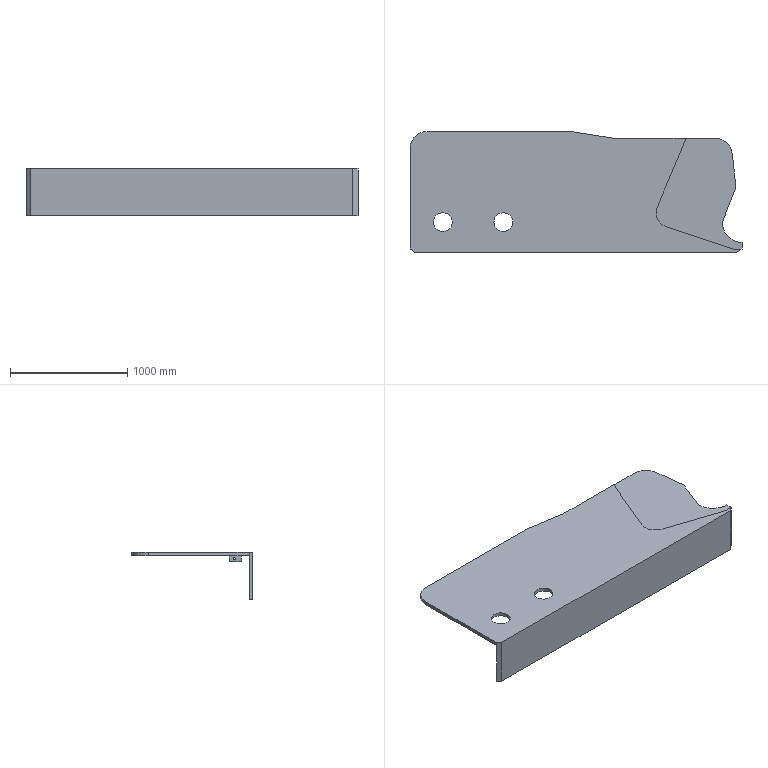Part | NX | features 掩护梁侧护板左 2 | 1 solid | 46 faces | box 2828 x 1030 x 405 mm | volume 109946345 mm3 | plane 36 | cylinder 10 | commonest cylinder face diameters 20 x4 160.33 x2 291.509 x2 250.37 x1 334.604 x1
STEP:
#1=CARTESIAN_POINT('',(589.52,-402.895,0.));
#2=VERTEX_POINT('',#1);
#3=CARTESIAN_POINT('',(589.52,-320.895,0.));
#4=VERTEX_POINT('',#3);
#5=CARTESIAN_POINT('',(589.52,-320.895,0.));
#6=DIRECTION('',(0.,1.,0.));
#7=VECTOR('',#6,1000.);
#8=LINE('',#5,#7);
#9=EDGE_CURVE('',#2,#4,#8,.T.);
#10=ORIENTED_EDGE('',*,*,#9,.F.);
#11=CARTESIAN_POINT('',(507.52,-402.895,0.));
#12=VERTEX_POINT('',#11);
#13=CARTESIAN_POINT('',(589.52,-402.895,0.));
#14=DIRECTION('',(1.,0.,0.));
#15=VECTOR('',#14,1000.);
#16=LINE('',#13,#15);
#17=EDGE_CURVE('',#12,#2,#16,.T.);
#18=ORIENTED_EDGE('',*,*,#17,.F.);
#19=CARTESIAN_POINT('',(507.52,-320.895,0.));
#20=VERTEX_POINT('',#19);
#21=CARTESIAN_POINT('',(507.52,-320.895,0.));
#22=DIRECTION('',(0.,-1.,0.));
#23=VECTOR('',#22,1000.);
#24=LINE('',#21,#23);
#25=EDGE_CURVE('',#20,#12,#24,.T.);
#26=ORIENTED_EDGE('',*,*,#25,.F.);
#27=CARTESIAN_POINT('',(482.52,-320.895,0.));
#28=VERTEX_POINT('',#27);
#29=CARTESIAN_POINT('',(482.52,-320.895,0.));
#30=DIRECTION('',(1.,0.,0.));
#31=VECTOR('',#30,1000.);
#32=LINE('',#29,#31);
#33=EDGE_CURVE('',#28,#20,#32,.T.);
#34=ORIENTED_EDGE('',*,*,#33,.F.);
#35=CARTESIAN_POINT('',(482.52,-422.895,0.));
#36=VERTEX_POINT('',#35);
#37=CARTESIAN_POINT('',(482.52,-422.895,0.));
#38=DIRECTION('',(0.,1.,0.));
#39=VECTOR('',#38,1000.);
#40=LINE('',#37,#39);
#41=EDGE_CURVE('',#36,#28,#40,.T.);
#42=ORIENTED_EDGE('',*,*,#41,.F.);
#43=CARTESIAN_POINT('',(614.52,-422.895,0.));
#44=VERTEX_POINT('',#43);
#45=CARTESIAN_POINT('',(614.52,-422.895,0.));
#46=DIRECTION('',(-1.,0.,0.));
#47=VECTOR('',#46,1000.);
#48=LINE('',#45,#47);
#49=EDGE_CURVE('',#44,#36,#48,.T.);
#50=ORIENTED_EDGE('',*,*,#49,.F.);
#51=CARTESIAN_POINT('',(614.52,-320.895,0.));
#52=VERTEX_POINT('',#51);
#53=CARTESIAN_POINT('',(614.52,-320.895,0.));
#54=DIRECTION('',(0.,-1.,0.));
#55=VECTOR('',#54,1000.);
#56=LINE('',#53,#55);
#57=EDGE_CURVE('',#52,#44,#56,.T.);
#58=ORIENTED_EDGE('',*,*,#57,.F.);
#59=CARTESIAN_POINT('',(589.52,-320.895,0.));
#60=DIRECTION('',(1.,0.,0.));
#61=VECTOR('',#60,1000.);
#62=LINE('',#59,#61);
#63=EDGE_CURVE('',#4,#52,#62,.T.);
#64=ORIENTED_EDGE('',*,*,#63,.F.);
#65=EDGE_LOOP('',(#10,#18,#26,#34,#42,#50,#58,#64));
#66=FACE_BOUND('',#65,.T.);
#67=CARTESIAN_POINT('',(-541.636,-260.046,0.));
#68=VERTEX_POINT('',#67);
#69=CARTESIAN_POINT('',(-621.801,-260.046,0.));
#70=DIRECTION('',(0.,0.,1.));
#71=DIRECTION('',(1.,0.,0.));
#72=AXIS2_PLACEMENT_3D('',#69,#70,#71);
#73=CIRCLE('',#72,80.165);
#74=EDGE_CURVE('',#68,#68,#73,.T.);
#75=ORIENTED_EDGE('',*,*,#74,.T.);
#76=EDGE_LOOP('',(#75));
#77=FACE_BOUND('',#76,.T.);
#78=CARTESIAN_POINT('',(-1056.636,-260.046,0.));
#79=VERTEX_POINT('',#78);
#80=CARTESIAN_POINT('',(-1136.801,-260.046,0.));
#81=DIRECTION('',(0.,0.,1.));
#82=DIRECTION('',(1.,0.,0.));
#83=AXIS2_PLACEMENT_3D('',#80,#81,#82);
#84=CIRCLE('',#83,80.165);
#85=EDGE_CURVE('',#79,#79,#84,.T.);
#86=ORIENTED_EDGE('',*,*,#85,.T.);
#87=EDGE_LOOP('',(#86));
#88=FACE_BOUND('',#87,.T.);
#89=CARTESIAN_POINT('',(-1416.65,-488.395,0.));
#90=VERTEX_POINT('',#89);
#91=CARTESIAN_POINT('',(1410.992,-488.395,0.));
#92=VERTEX_POINT('',#91);
#93=CARTESIAN_POINT('',(1410.992,-488.395,0.));
#94=DIRECTION('',(1.,0.,0.));
#95=VECTOR('',#94,1000.);
#96=LINE('',#93,#95);
#97=EDGE_CURVE('',#90,#92,#96,.T.);
#98=ORIENTED_EDGE('',*,*,#97,.F.);
#99=CARTESIAN_POINT('',(-1416.65,366.699,0.));
#100=VERTEX_POINT('',#99);
#101=CARTESIAN_POINT('',(-1416.65,366.699,0.));
#102=DIRECTION('',(0.,-1.,0.));
#103=VECTOR('',#102,1000.);
#104=LINE('',#101,#103);
#105=EDGE_CURVE('',#100,#90,#104,.T.);
#106=ORIENTED_EDGE('',*,*,#105,.F.);
#107=CARTESIAN_POINT('',(-1270.895,512.454,0.));
#108=VERTEX_POINT('',#107);
#109=CARTESIAN_POINT('',(-1270.895,366.699,0.));
#110=DIRECTION('',(0.,0.,1.));
#111=DIRECTION('',(1.,0.,0.));
#112=AXIS2_PLACEMENT_3D('',#109,#110,#111);
#113=CIRCLE('',#112,145.755);
#114=EDGE_CURVE('',#108,#100,#113,.T.);
#115=ORIENTED_EDGE('',*,*,#114,.F.);
#116=CARTESIAN_POINT('',(-51.414,512.454,0.));
#117=VERTEX_POINT('',#116);
#118=CARTESIAN_POINT('',(-51.414,512.454,0.));
#119=DIRECTION('',(-1.,0.,0.));
#120=VECTOR('',#119,1000.);
#121=LINE('',#118,#120);
#122=EDGE_CURVE('',#117,#108,#121,.T.);
#123=ORIENTED_EDGE('',*,*,#122,.F.);
#124=CARTESIAN_POINT('',(324.663,454.152,0.));
#125=VERTEX_POINT('',#124);
#126=CARTESIAN_POINT('',(324.663,454.152,0.));
#127=DIRECTION('',(-0.9882,0.1532,0.));
#128=VECTOR('',#127,1000.);
#129=LINE('',#126,#128);
#130=EDGE_CURVE('',#125,#117,#129,.T.);
#131=ORIENTED_EDGE('',*,*,#130,.F.);
#132=CARTESIAN_POINT('',(1182.944,454.152,0.));
#133=VERTEX_POINT('',#132);
#134=CARTESIAN_POINT('',(935.041,454.152,0.));
#135=DIRECTION('',(-1.,0.,0.));
#136=VECTOR('',#135,1000.);
#137=LINE('',#134,#136);
#138=EDGE_CURVE('',#133,#125,#137,.T.);
#139=ORIENTED_EDGE('',*,*,#138,.F.);
#140=CARTESIAN_POINT('',(1327.809,324.481,0.));
#141=VERTEX_POINT('',#140);
#142=CARTESIAN_POINT('',(1182.944,308.397,0.));
#143=DIRECTION('',(0.,0.,1.));
#144=DIRECTION('',(1.,0.,0.));
#145=AXIS2_PLACEMENT_3D('',#142,#143,#144);
#146=CIRCLE('',#145,145.755);
#147=EDGE_CURVE('',#141,#133,#146,.T.);
#148=ORIENTED_EDGE('',*,*,#147,.F.);
#149=CARTESIAN_POINT('',(1359.76,36.697,0.));
#150=VERTEX_POINT('',#149);
#151=CARTESIAN_POINT('',(1359.76,36.697,0.));
#152=DIRECTION('',(-0.1103,0.9939,0.));
#153=VECTOR('',#152,1000.);
#154=LINE('',#151,#153);
#155=EDGE_CURVE('',#150,#141,#154,.T.);
#156=ORIENTED_EDGE('',*,*,#155,.F.);
#157=CARTESIAN_POINT('',(1243.69,-260.046,0.));
#158=VERTEX_POINT('',#157);
#159=CARTESIAN_POINT('',(1243.69,-260.046,0.));
#160=DIRECTION('',(0.3643,0.9313,0.));
#161=VECTOR('',#160,1000.);
#162=LINE('',#159,#161);
#163=EDGE_CURVE('',#158,#150,#162,.T.);
#164=ORIENTED_EDGE('',*,*,#163,.F.);
#165=CARTESIAN_POINT('',(1410.992,-432.474,0.));
#166=VERTEX_POINT('',#165);
#167=CARTESIAN_POINT('',(1410.913,-265.172,0.));
#168=DIRECTION('',(0.,0.,-1.));
#169=DIRECTION('',(1.,0.,0.));
#170=AXIS2_PLACEMENT_3D('',#167,#168,#169);
#171=CIRCLE('',#170,167.302);
#172=EDGE_CURVE('',#166,#158,#171,.T.);
#173=ORIENTED_EDGE('',*,*,#172,.F.);
#174=CARTESIAN_POINT('',(1410.992,-488.395,0.));
#175=DIRECTION('',(0.,1.,0.));
#176=VECTOR('',#175,1000.);
#177=LINE('',#174,#176);
#178=EDGE_CURVE('',#92,#166,#177,.T.);
#179=ORIENTED_EDGE('',*,*,#178,.F.);
#180=EDGE_LOOP('',(#98,#106,#115,#123,#131,#139,#148,#156,#164,#173,#179));
#181=FACE_BOUND('',#180,.T.);
#182=CARTESIAN_POINT('',(-870.51,-402.895,0.));
#183=VERTEX_POINT('',#182);
#184=CARTESIAN_POINT('',(-870.51,-320.895,0.));
#185=VERTEX_POINT('',#184);
#186=CARTESIAN_POINT('',(-870.51,-320.895,0.));
#187=DIRECTION('',(0.,1.,0.));
#188=VECTOR('',#187,1000.);
#189=LINE('',#186,#188);
#190=EDGE_CURVE('',#183,#185,#189,.T.);
#191=ORIENTED_EDGE('',*,*,#190,.F.);
#192=CARTESIAN_POINT('',(-952.51,-402.895,0.));
#193=VERTEX_POINT('',#192);
#194=CARTESIAN_POINT('',(-870.51,-402.895,0.));
#195=DIRECTION('',(1.,0.,0.));
#196=VECTOR('',#195,1000.);
#197=LINE('',#194,#196);
#198=EDGE_CURVE('',#193,#183,#197,.T.);
#199=ORIENTED_EDGE('',*,*,#198,.F.);
#200=CARTESIAN_POINT('',(-952.51,-320.895,0.));
#201=VERTEX_POINT('',#200);
#202=CARTESIAN_POINT('',(-952.51,-320.895,0.));
#203=DIRECTION('',(0.,-1.,0.));
#204=VECTOR('',#203,1000.);
#205=LINE('',#202,#204);
#206=EDGE_CURVE('',#201,#193,#205,.T.);
#207=ORIENTED_EDGE('',*,*,#206,.F.);
#208=CARTESIAN_POINT('',(-977.51,-320.895,0.));
#209=VERTEX_POINT('',#208);
#210=CARTESIAN_POINT('',(-977.51,-320.895,0.));
#211=DIRECTION('',(1.,0.,0.));
#212=VECTOR('',#211,1000.);
#213=LINE('',#210,#212);
#214=EDGE_CURVE('',#209,#201,#213,.T.);
#215=ORIENTED_EDGE('',*,*,#214,.F.);
#216=CARTESIAN_POINT('',(-977.51,-422.895,0.));
#217=VERTEX_POINT('',#216);
#218=CARTESIAN_POINT('',(-977.51,-422.895,0.));
#219=DIRECTION('',(0.,1.,0.));
#220=VECTOR('',#219,1000.);
#221=LINE('',#218,#220);
#222=EDGE_CURVE('',#217,#209,#221,.T.);
#223=ORIENTED_EDGE('',*,*,#222,.F.);
#224=CARTESIAN_POINT('',(-845.51,-422.895,0.));
#225=VERTEX_POINT('',#224);
#226=CARTESIAN_POINT('',(-845.51,-422.895,0.));
#227=DIRECTION('',(-1.,0.,0.));
#228=VECTOR('',#227,1000.);
#229=LINE('',#226,#228);
#230=EDGE_CURVE('',#225,#217,#229,.T.);
#231=ORIENTED_EDGE('',*,*,#230,.F.);
#232=CARTESIAN_POINT('',(-845.51,-320.895,0.));
#233=VERTEX_POINT('',#232);
#234=CARTESIAN_POINT('',(-845.51,-320.895,0.));
#235=DIRECTION('',(0.,-1.,0.));
#236=VECTOR('',#235,1000.);
#237=LINE('',#234,#236);
#238=EDGE_CURVE('',#233,#225,#237,.T.);
#239=ORIENTED_EDGE('',*,*,#238,.F.);
#240=CARTESIAN_POINT('',(-870.51,-320.895,0.));
#241=DIRECTION('',(1.,0.,0.));
#242=VECTOR('',#241,1000.);
#243=LINE('',#240,#242);
#244=EDGE_CURVE('',#185,#233,#243,.T.);
#245=ORIENTED_EDGE('',*,*,#244,.F.);
#246=EDGE_LOOP('',(#191,#199,#207,#215,#223,#231,#239,#245));
#247=FACE_BOUND('',#246,.T.);
#248=CARTESIAN_POINT('',(-1270.895,366.699,0.));
#249=DIRECTION('',(0.,0.,1.));
#250=DIRECTION('',(1.,0.,0.));
#251=AXIS2_PLACEMENT_3D('',#248,#249,#250);
#252=PLANE('',#251);
#253=ADVANCED_FACE('',(#66,#77,#88,#181,#247),#252,.F.);
#254=CARTESIAN_POINT('',(1410.992,-488.395,25.));
#255=VERTEX_POINT('',#254);
#256=CARTESIAN_POINT('',(1410.992,-432.474,25.));
#257=VERTEX_POINT('',#256);
#258=CARTESIAN_POINT('',(1410.992,-488.395,25.));
#259=DIRECTION('',(0.,1.,0.));
#260=VECTOR('',#259,1000.);
#261=LINE('',#258,#260);
#262=EDGE_CURVE('',#255,#257,#261,.T.);
#263=ORIENTED_EDGE('',*,*,#262,.F.);
#264=CARTESIAN_POINT('',(1410.992,-488.395,30.));
#265=DIRECTION('',(0.,0.,-1.));
#266=VECTOR('',#265,1000.);
#267=LINE('',#264,#266);
#268=EDGE_CURVE('',#255,#92,#267,.T.);
#269=ORIENTED_EDGE('',*,*,#268,.T.);
#270=ORIENTED_EDGE('',*,*,#178,.T.);
#271=CARTESIAN_POINT('',(1410.992,-432.474,30.));
#272=DIRECTION('',(0.,0.,-1.));
#273=VECTOR('',#272,1000.);
#274=LINE('',#271,#273);
#275=EDGE_CURVE('',#257,#166,#274,.T.);
#276=ORIENTED_EDGE('',*,*,#275,.F.);
#277=EDGE_LOOP('',(#263,#269,#270,#276));
#278=FACE_BOUND('',#277,.T.);
#279=CARTESIAN_POINT('',(1410.992,-488.395,30.));
#280=DIRECTION('',(-1.,0.,0.));
#281=DIRECTION('',(0.,0.,1.));
#282=AXIS2_PLACEMENT_3D('',#279,#280,#281);
#283=PLANE('',#282);
#284=ADVANCED_FACE('',(#278),#283,.F.);
#285=CARTESIAN_POINT('',(1243.69,-260.046,25.));
#286=VERTEX_POINT('',#285);
#287=CARTESIAN_POINT('',(1410.913,-265.172,25.));
#288=DIRECTION('',(0.,0.,1.));
#289=DIRECTION('',(1.,0.,0.));
#290=AXIS2_PLACEMENT_3D('',#287,#288,#289);
#291=CIRCLE('',#290,167.302);
#292=EDGE_CURVE('',#257,#286,#291,.F.);
#293=ORIENTED_EDGE('',*,*,#292,.F.);
#294=ORIENTED_EDGE('',*,*,#275,.T.);
#295=ORIENTED_EDGE('',*,*,#172,.T.);
#296=CARTESIAN_POINT('',(1243.69,-260.046,30.));
#297=DIRECTION('',(0.,0.,-1.));
#298=VECTOR('',#297,1000.);
#299=LINE('',#296,#298);
#300=EDGE_CURVE('',#286,#158,#299,.T.);
#301=ORIENTED_EDGE('',*,*,#300,.F.);
#302=EDGE_LOOP('',(#293,#294,#295,#301));
#303=FACE_BOUND('',#302,.T.);
#304=CARTESIAN_POINT('',(1410.913,-265.172,30.));
#305=DIRECTION('',(0.,0.,-1.));
#306=DIRECTION('',(-1.,0.,0.));
#307=AXIS2_PLACEMENT_3D('',#304,#305,#306);
#308=CYLINDRICAL_SURFACE('',#307,167.302);
#309=ADVANCED_FACE('',(#303),#308,.F.);
#310=CARTESIAN_POINT('',(1359.76,36.697,25.));
#311=VERTEX_POINT('',#310);
#312=CARTESIAN_POINT('',(1243.69,-260.046,25.));
#313=DIRECTION('',(0.3643,0.9313,0.));
#314=VECTOR('',#313,1000.);
#315=LINE('',#312,#314);
#316=EDGE_CURVE('',#286,#311,#315,.T.);
#317=ORIENTED_EDGE('',*,*,#316,.F.);
#318=ORIENTED_EDGE('',*,*,#300,.T.);
#319=ORIENTED_EDGE('',*,*,#163,.T.);
#320=CARTESIAN_POINT('',(1359.76,36.697,30.));
#321=DIRECTION('',(0.,0.,-1.));
#322=VECTOR('',#321,1000.);
#323=LINE('',#320,#322);
#324=EDGE_CURVE('',#311,#150,#323,.T.);
#325=ORIENTED_EDGE('',*,*,#324,.F.);
#326=EDGE_LOOP('',(#317,#318,#319,#325));
#327=FACE_BOUND('',#326,.T.);
#328=CARTESIAN_POINT('',(1243.69,-260.046,30.));
#329=DIRECTION('',(-0.9313,0.3643,0.));
#330=DIRECTION('',(-0.3643,-0.9313,0.));
#331=AXIS2_PLACEMENT_3D('',#328,#329,#330);
#332=PLANE('',#331);
#333=ADVANCED_FACE('',(#327),#332,.F.);
#334=CARTESIAN_POINT('',(1327.809,324.481,25.));
#335=VERTEX_POINT('',#334);
#336=CARTESIAN_POINT('',(1359.76,36.697,25.));
#337=DIRECTION('',(-0.1103,0.9939,0.));
#338=VECTOR('',#337,1000.);
#339=LINE('',#336,#338);
#340=EDGE_CURVE('',#311,#335,#339,.T.);
#341=ORIENTED_EDGE('',*,*,#340,.F.);
#342=ORIENTED_EDGE('',*,*,#324,.T.);
#343=ORIENTED_EDGE('',*,*,#155,.T.);
#344=CARTESIAN_POINT('',(1327.809,324.481,30.));
#345=DIRECTION('',(0.,0.,-1.));
#346=VECTOR('',#345,1000.);
#347=LINE('',#344,#346);
#348=EDGE_CURVE('',#335,#141,#347,.T.);
#349=ORIENTED_EDGE('',*,*,#348,.F.);
#350=EDGE_LOOP('',(#341,#342,#343,#349));
#351=FACE_BOUND('',#350,.T.);
#352=CARTESIAN_POINT('',(1359.76,36.697,30.));
#353=DIRECTION('',(-0.9939,-0.1103,0.));
#354=DIRECTION('',(0.1103,-0.9939,0.));
#355=AXIS2_PLACEMENT_3D('',#352,#353,#354);
#356=PLANE('',#355);
#357=ADVANCED_FACE('',(#351),#356,.F.);
#358=CARTESIAN_POINT('',(1182.944,454.152,25.));
#359=VERTEX_POINT('',#358);
#360=CARTESIAN_POINT('',(1182.944,308.397,25.));
#361=DIRECTION('',(0.,0.,1.));
#362=DIRECTION('',(1.,0.,0.));
#363=AXIS2_PLACEMENT_3D('',#360,#361,#362);
#364=CIRCLE('',#363,145.755);
#365=EDGE_CURVE('',#335,#359,#364,.T.);
#366=ORIENTED_EDGE('',*,*,#365,.F.);
#367=ORIENTED_EDGE('',*,*,#348,.T.);
#368=ORIENTED_EDGE('',*,*,#147,.T.);
#369=CARTESIAN_POINT('',(1182.944,454.152,30.));
#370=DIRECTION('',(0.,0.,-1.));
#371=VECTOR('',#370,1000.);
#372=LINE('',#369,#371);
#373=EDGE_CURVE('',#359,#133,#372,.T.);
#374=ORIENTED_EDGE('',*,*,#373,.F.);
#375=EDGE_LOOP('',(#366,#367,#368,#374));
#376=FACE_BOUND('',#375,.T.);
#377=CARTESIAN_POINT('',(1182.944,308.397,30.));
#378=DIRECTION('',(0.,0.,-1.));
#379=DIRECTION('',(-1.,0.,0.));
#380=AXIS2_PLACEMENT_3D('',#377,#378,#379);
#381=CYLINDRICAL_SURFACE('',#380,145.755);
#382=ADVANCED_FACE('',(#376),#381,.T.);
#383=CARTESIAN_POINT('',(1337.166,-488.395,30.));
#384=VERTEX_POINT('',#383);
#385=CARTESIAN_POINT('',(1410.992,-488.395,30.));
#386=VERTEX_POINT('',#385);
#387=CARTESIAN_POINT('',(1337.166,-488.395,30.));
#388=DIRECTION('',(1.,0.,0.));
#389=VECTOR('',#388,1000.);
#390=LINE('',#387,#389);
#391=EDGE_CURVE('',#384,#386,#390,.T.);
#392=ORIENTED_EDGE('',*,*,#391,.F.);
#393=CARTESIAN_POINT('',(764.685,-299.875,30.));
#394=VERTEX_POINT('',#393);
#395=CARTESIAN_POINT('',(764.685,-299.875,30.));
#396=DIRECTION('',(0.9498,-0.3128,0.));
#397=VECTOR('',#396,1000.);
#398=LINE('',#395,#397);
#399=EDGE_CURVE('',#394,#384,#398,.T.);
#400=ORIENTED_EDGE('',*,*,#399,.F.);
#401=CARTESIAN_POINT('',(688.438,-132.458,30.));
#402=VERTEX_POINT('',#401);
#403=CARTESIAN_POINT('',(803.841,-180.971,30.));
#404=DIRECTION('',(0.,0.,1.));
#405=DIRECTION('',(1.,0.,0.));
#406=AXIS2_PLACEMENT_3D('',#403,#404,#405);
#407=CIRCLE('',#406,125.185);
#408=EDGE_CURVE('',#402,#394,#407,.T.);
#409=ORIENTED_EDGE('',*,*,#408,.F.);
#410=CARTESIAN_POINT('',(935.041,454.152,30.));
#411=VERTEX_POINT('',#410);
#412=CARTESIAN_POINT('',(935.041,454.152,30.));
#413=DIRECTION('',(-0.3875,-0.9219,0.));
#414=VECTOR('',#413,1000.);
#415=LINE('',#412,#414);
#416=EDGE_CURVE('',#411,#402,#415,.T.);
#417=ORIENTED_EDGE('',*,*,#416,.F.);
#418=CARTESIAN_POINT('',(324.663,454.152,30.));
#419=VERTEX_POINT('',#418);
#420=CARTESIAN_POINT('',(1182.944,454.152,30.));
#421=DIRECTION('',(-1.,0.,0.));
#422=VECTOR('',#421,1000.);
#423=LINE('',#420,#422);
#424=EDGE_CURVE('',#411,#419,#423,.T.);
#425=ORIENTED_EDGE('',*,*,#424,.T.);
#426=CARTESIAN_POINT('',(-51.414,512.454,30.));
#427=VERTEX_POINT('',#426);
#428=CARTESIAN_POINT('',(324.663,454.152,30.));
#429=DIRECTION('',(-0.9882,0.1532,0.));
#430=VECTOR('',#429,1000.);
#431=LINE('',#428,#430);
#432=EDGE_CURVE('',#419,#427,#431,.T.);
#433=ORIENTED_EDGE('',*,*,#432,.T.);
#434=CARTESIAN_POINT('',(-1270.895,512.454,30.));
#435=VERTEX_POINT('',#434);
#436=CARTESIAN_POINT('',(-51.414,512.454,30.));
#437=DIRECTION('',(-1.,0.,0.));
#438=VECTOR('',#437,1000.);
#439=LINE('',#436,#438);
#440=EDGE_CURVE('',#427,#435,#439,.T.);
#441=ORIENTED_EDGE('',*,*,#440,.T.);
#442=CARTESIAN_POINT('',(-1416.65,366.699,30.));
#443=VERTEX_POINT('',#442);
#444=CARTESIAN_POINT('',(-1270.895,366.699,30.));
#445=DIRECTION('',(0.,0.,1.));
#446=DIRECTION('',(1.,0.,0.));
#447=AXIS2_PLACEMENT_3D('',#444,#445,#446);
#448=CIRCLE('',#447,145.755);
#449=EDGE_CURVE('',#435,#443,#448,.T.);
#450=ORIENTED_EDGE('',*,*,#449,.T.);
#451=CARTESIAN_POINT('',(-1416.65,-488.395,30.));
#452=VERTEX_POINT('',#451);
#453=CARTESIAN_POINT('',(-1416.65,366.699,30.));
#454=DIRECTION('',(0.,-1.,0.));
#455=VECTOR('',#454,1000.);
#456=LINE('',#453,#455);
#457=EDGE_CURVE('',#443,#452,#456,.T.);
#458=ORIENTED_EDGE('',*,*,#457,.T.);
#459=CARTESIAN_POINT('',(-1381.422,-517.546,30.));
#460=VERTEX_POINT('',#459);
#461=CARTESIAN_POINT('',(-1381.422,-517.546,30.));
#462=DIRECTION('',(0.7704,-0.6375,0.));
#463=VECTOR('',#462,1000.);
#464=LINE('',#461,#463);
#465=EDGE_CURVE('',#452,#460,#464,.T.);
#466=ORIENTED_EDGE('',*,*,#465,.T.);
#467=CARTESIAN_POINT('',(1367.913,-517.546,30.));
#468=VERTEX_POINT('',#467);
#469=CARTESIAN_POINT('',(1367.913,-517.546,30.));
#470=DIRECTION('',(1.,0.,0.));
#471=VECTOR('',#470,1000.);
#472=LINE('',#469,#471);
#473=EDGE_CURVE('',#460,#468,#472,.T.);
#474=ORIENTED_EDGE('',*,*,#473,.T.);
#475=CARTESIAN_POINT('',(1410.992,-488.395,30.));
#476=DIRECTION('',(0.8282,0.5604,0.));
#477=VECTOR('',#476,1000.);
#478=LINE('',#475,#477);
#479=EDGE_CURVE('',#468,#386,#478,.T.);
#480=ORIENTED_EDGE('',*,*,#479,.T.);
#481=EDGE_LOOP('',(#392,#400,#409,#417,#425,#433,#441,#450,#458,#466,#474,#480));
#482=FACE_BOUND('',#481,.T.);
#483=CARTESIAN_POINT('',(-1056.636,-260.046,30.));
#484=VERTEX_POINT('',#483);
#485=CARTESIAN_POINT('',(-1136.801,-260.046,30.));
#486=DIRECTION('',(0.,0.,1.));
#487=DIRECTION('',(1.,0.,0.));
#488=AXIS2_PLACEMENT_3D('',#485,#486,#487);
#489=CIRCLE('',#488,80.165);
#490=EDGE_CURVE('',#484,#484,#489,.T.);
#491=ORIENTED_EDGE('',*,*,#490,.F.);
#492=EDGE_LOOP('',(#491));
#493=FACE_BOUND('',#492,.T.);
#494=CARTESIAN_POINT('',(-541.636,-260.046,30.));
#495=VERTEX_POINT('',#494);
#496=CARTESIAN_POINT('',(-621.801,-260.046,30.));
#497=DIRECTION('',(0.,0.,1.));
#498=DIRECTION('',(1.,0.,0.));
#499=AXIS2_PLACEMENT_3D('',#496,#497,#498);
#500=CIRCLE('',#499,80.165);
#501=EDGE_CURVE('',#495,#495,#500,.T.);
#502=ORIENTED_EDGE('',*,*,#501,.F.);
#503=EDGE_LOOP('',(#502));
#504=FACE_BOUND('',#503,.T.);
#505=CARTESIAN_POINT('',(-1270.895,366.699,30.));
#506=DIRECTION('',(0.,0.,1.));
#507=DIRECTION('',(1.,0.,0.));
#508=AXIS2_PLACEMENT_3D('',#505,#506,#507);
#509=PLANE('',#508);
#510=ADVANCED_FACE('',(#482,#493,#504),#509,.T.);
#511=ORIENTED_EDGE('',*,*,#114,.T.);
#512=CARTESIAN_POINT('',(-1416.65,366.699,30.));
#513=DIRECTION('',(0.,0.,-1.));
#514=VECTOR('',#513,1000.);
#515=LINE('',#512,#514);
#516=EDGE_CURVE('',#443,#100,#515,.T.);
#517=ORIENTED_EDGE('',*,*,#516,.F.);
#518=ORIENTED_EDGE('',*,*,#449,.F.);
#519=CARTESIAN_POINT('',(-1270.895,512.454,30.));
#520=DIRECTION('',(0.,0.,-1.));
#521=VECTOR('',#520,1000.);
#522=LINE('',#519,#521);
#523=EDGE_CURVE('',#435,#108,#522,.T.);
#524=ORIENTED_EDGE('',*,*,#523,.T.);
#525=EDGE_LOOP('',(#511,#517,#518,#524));
#526=FACE_BOUND('',#525,.T.);
#527=CARTESIAN_POINT('',(-1270.895,366.699,30.));
#528=DIRECTION('',(0.,0.,-1.));
#529=DIRECTION('',(-1.,0.,0.));
#530=AXIS2_PLACEMENT_3D('',#527,#528,#529);
#531=CYLINDRICAL_SURFACE('',#530,145.755);
#532=ADVANCED_FACE('',(#526),#531,.T.);
#533=ORIENTED_EDGE('',*,*,#105,.T.);
#534=CARTESIAN_POINT('',(-1416.65,-488.395,30.));
#535=DIRECTION('',(0.,0.,-1.));
#536=VECTOR('',#535,1000.);
#537=LINE('',#534,#536);
#538=EDGE_CURVE('',#452,#90,#537,.T.);
#539=ORIENTED_EDGE('',*,*,#538,.F.);
#540=ORIENTED_EDGE('',*,*,#457,.F.);
#541=ORIENTED_EDGE('',*,*,#516,.T.);
#542=EDGE_LOOP('',(#533,#539,#540,#541));
#543=FACE_BOUND('',#542,.T.);
#544=CARTESIAN_POINT('',(-1416.65,366.699,30.));
#545=DIRECTION('',(1.,0.,0.));
#546=DIRECTION('',(0.,0.,-1.));
#547=AXIS2_PLACEMENT_3D('',#544,#545,#546);
#548=PLANE('',#547);
#549=ADVANCED_FACE('',(#543),#548,.F.);
#550=ORIENTED_EDGE('',*,*,#538,.T.);
#551=CARTESIAN_POINT('',(-1416.65,-488.395,-375.));
#552=VERTEX_POINT('',#551);
#553=CARTESIAN_POINT('',(-1416.65,-488.395,-375.));
#554=DIRECTION('',(0.,0.,1.));
#555=VECTOR('',#554,1000.);
#556=LINE('',#553,#555);
#557=EDGE_CURVE('',#552,#90,#556,.T.);
#558=ORIENTED_EDGE('',*,*,#557,.F.);
#559=CARTESIAN_POINT('',(-1381.422,-517.546,-375.));
#560=VERTEX_POINT('',#559);
#561=CARTESIAN_POINT('',(-1416.65,-488.395,-375.));
#562=DIRECTION('',(-0.7704,0.6375,0.));
#563=VECTOR('',#562,1000.);
#564=LINE('',#561,#563);
#565=EDGE_CURVE('',#560,#552,#564,.T.);
#566=ORIENTED_EDGE('',*,*,#565,.F.);
#567=CARTESIAN_POINT('',(-1381.422,-517.546,30.));
#568=DIRECTION('',(0.,0.,-1.));
#569=VECTOR('',#568,1000.);
#570=LINE('',#567,#569);
#571=EDGE_CURVE('',#460,#560,#570,.T.);
#572=ORIENTED_EDGE('',*,*,#571,.F.);
#573=ORIENTED_EDGE('',*,*,#465,.F.);
#574=EDGE_LOOP('',(#550,#558,#566,#572,#573));
#575=FACE_BOUND('',#574,.T.);
#576=CARTESIAN_POINT('',(-1381.422,-517.546,30.));
#577=DIRECTION('',(0.6375,0.7704,0.));
#578=DIRECTION('',(-0.7704,0.6375,0.));
#579=AXIS2_PLACEMENT_3D('',#576,#577,#578);
#580=PLANE('',#579);
#581=ADVANCED_FACE('',(#575),#580,.F.);
#582=ORIENTED_EDGE('',*,*,#571,.T.);
#583=CARTESIAN_POINT('',(1367.913,-517.546,-375.));
#584=VERTEX_POINT('',#583);
#585=CARTESIAN_POINT('',(-1381.422,-517.546,-375.));
#586=DIRECTION('',(-1.,0.,0.));
#587=VECTOR('',#586,1000.);
#588=LINE('',#585,#587);
#589=EDGE_CURVE('',#584,#560,#588,.T.);
#590=ORIENTED_EDGE('',*,*,#589,.F.);
#591=CARTESIAN_POINT('',(1367.913,-517.546,30.));
#592=DIRECTION('',(0.,0.,-1.));
#593=VECTOR('',#592,1000.);
#594=LINE('',#591,#593);
#595=EDGE_CURVE('',#468,#584,#594,.T.);
#596=ORIENTED_EDGE('',*,*,#595,.F.);
#597=ORIENTED_EDGE('',*,*,#473,.F.);
#598=EDGE_LOOP('',(#582,#590,#596,#597));
#599=FACE_BOUND('',#598,.T.);
#600=CARTESIAN_POINT('',(1367.913,-517.546,30.));
#601=DIRECTION('',(0.,1.,0.));
#602=DIRECTION('',(-1.,0.,0.));
#603=AXIS2_PLACEMENT_3D('',#600,#601,#602);
#604=PLANE('',#603);
#605=ADVANCED_FACE('',(#599),#604,.F.);
#606=ORIENTED_EDGE('',*,*,#595,.T.);
#607=CARTESIAN_POINT('',(1410.992,-488.395,-375.));
#608=VERTEX_POINT('',#607);
#609=CARTESIAN_POINT('',(1367.913,-517.546,-375.));
#610=DIRECTION('',(-0.8282,-0.5604,0.));
#611=VECTOR('',#610,1000.);
#612=LINE('',#609,#611);
#613=EDGE_CURVE('',#608,#584,#612,.T.);
#614=ORIENTED_EDGE('',*,*,#613,.F.);
#615=CARTESIAN_POINT('',(1410.992,-488.395,-375.));
#616=DIRECTION('',(0.,0.,1.));
#617=VECTOR('',#616,1000.);
#618=LINE('',#615,#617);
#619=EDGE_CURVE('',#608,#92,#618,.T.);
#620=ORIENTED_EDGE('',*,*,#619,.T.);
#621=ORIENTED_EDGE('',*,*,#268,.F.);
#622=CARTESIAN_POINT('',(1410.992,-488.395,30.));
#623=DIRECTION('',(0.,0.,-1.));
#624=VECTOR('',#623,1000.);
#625=LINE('',#622,#624);
#626=EDGE_CURVE('',#386,#255,#625,.T.);
#627=ORIENTED_EDGE('',*,*,#626,.F.);
#628=ORIENTED_EDGE('',*,*,#479,.F.);
#629=EDGE_LOOP('',(#606,#614,#620,#621,#627,#628));
#630=FACE_BOUND('',#629,.T.);
#631=CARTESIAN_POINT('',(1410.992,-488.395,30.));
#632=DIRECTION('',(-0.5604,0.8282,0.));
#633=DIRECTION('',(-0.8282,-0.5604,0.));
#634=AXIS2_PLACEMENT_3D('',#631,#632,#633);
#635=PLANE('',#634);
#636=ADVANCED_FACE('',(#630),#635,.F.);
#637=ORIENTED_EDGE('',*,*,#424,.F.);
#638=CARTESIAN_POINT('',(935.041,454.152,25.));
#639=VERTEX_POINT('',#638);
#640=CARTESIAN_POINT('',(935.041,454.152,25.));
#641=DIRECTION('',(0.,0.,1.));
#642=VECTOR('',#641,1000.);
#643=LINE('',#640,#642);
#644=EDGE_CURVE('',#639,#411,#643,.T.);
#645=ORIENTED_EDGE('',*,*,#644,.F.);
#646=CARTESIAN_POINT('',(935.041,454.152,25.));
#647=DIRECTION('',(-1.,0.,0.));
#648=VECTOR('',#647,1000.);
#649=LINE('',#646,#648);
#650=EDGE_CURVE('',#359,#639,#649,.T.);
#651=ORIENTED_EDGE('',*,*,#650,.F.);
#652=ORIENTED_EDGE('',*,*,#373,.T.);
#653=ORIENTED_EDGE('',*,*,#138,.T.);
#654=CARTESIAN_POINT('',(324.663,454.152,30.));
#655=DIRECTION('',(0.,0.,-1.));
#656=VECTOR('',#655,1000.);
#657=LINE('',#654,#656);
#658=EDGE_CURVE('',#419,#125,#657,.T.);
#659=ORIENTED_EDGE('',*,*,#658,.F.);
#660=EDGE_LOOP('',(#637,#645,#651,#652,#653,#659));
#661=FACE_BOUND('',#660,.T.);
#662=CARTESIAN_POINT('',(935.041,454.152,30.));
#663=DIRECTION('',(0.,-1.,0.));
#664=DIRECTION('',(1.,0.,0.));
#665=AXIS2_PLACEMENT_3D('',#662,#663,#664);
#666=PLANE('',#665);
#667=ADVANCED_FACE('',(#661),#666,.F.);
#668=ORIENTED_EDGE('',*,*,#130,.T.);
#669=CARTESIAN_POINT('',(-51.414,512.454,30.));
#670=DIRECTION('',(0.,0.,-1.));
#671=VECTOR('',#670,1000.);
#672=LINE('',#669,#671);
#673=EDGE_CURVE('',#427,#117,#672,.T.);
#674=ORIENTED_EDGE('',*,*,#673,.F.);
#675=ORIENTED_EDGE('',*,*,#432,.F.);
#676=ORIENTED_EDGE('',*,*,#658,.T.);
#677=EDGE_LOOP('',(#668,#674,#675,#676));
#678=FACE_BOUND('',#677,.T.);
#679=CARTESIAN_POINT('',(324.663,454.152,30.));
#680=DIRECTION('',(-0.1532,-0.9882,0.));
#681=DIRECTION('',(0.9882,-0.1532,0.));
#682=AXIS2_PLACEMENT_3D('',#679,#680,#681);
#683=PLANE('',#682);
#684=ADVANCED_FACE('',(#678),#683,.F.);
#685=ORIENTED_EDGE('',*,*,#122,.T.);
#686=ORIENTED_EDGE('',*,*,#523,.F.);
#687=ORIENTED_EDGE('',*,*,#440,.F.);
#688=ORIENTED_EDGE('',*,*,#673,.T.);
#689=EDGE_LOOP('',(#685,#686,#687,#688));
#690=FACE_BOUND('',#689,.T.);
#691=CARTESIAN_POINT('',(-51.414,512.454,30.));
#692=DIRECTION('',(0.,-1.,0.));
#693=DIRECTION('',(0.,0.,-1.));
#694=AXIS2_PLACEMENT_3D('',#691,#692,#693);
#695=PLANE('',#694);
#696=ADVANCED_FACE('',(#690),#695,.F.);
#697=ORIENTED_EDGE('',*,*,#490,.T.);
#698=EDGE_LOOP('',(#697));
#699=FACE_BOUND('',#698,.T.);
#700=ORIENTED_EDGE('',*,*,#85,.F.);
#701=EDGE_LOOP('',(#700));
#702=FACE_BOUND('',#701,.T.);
#703=CARTESIAN_POINT('',(-1136.801,-260.046,30.));
#704=DIRECTION('',(0.,0.,-1.));
#705=DIRECTION('',(-1.,0.,0.));
#706=AXIS2_PLACEMENT_3D('',#703,#704,#705);
#707=CYLINDRICAL_SURFACE('',#706,80.165);
#708=ADVANCED_FACE('',(#699,#702),#707,.F.);
#709=ORIENTED_EDGE('',*,*,#501,.T.);
#710=EDGE_LOOP('',(#709));
#711=FACE_BOUND('',#710,.T.);
#712=ORIENTED_EDGE('',*,*,#74,.F.);
#713=EDGE_LOOP('',(#712));
#714=FACE_BOUND('',#713,.T.);
#715=CARTESIAN_POINT('',(-621.801,-260.046,30.));
#716=DIRECTION('',(0.,0.,-1.));
#717=DIRECTION('',(-1.,0.,0.));
#718=AXIS2_PLACEMENT_3D('',#715,#716,#717);
#719=CYLINDRICAL_SURFACE('',#718,80.165);
#720=ADVANCED_FACE('',(#711,#714),#719,.F.);
#721=ORIENTED_EDGE('',*,*,#292,.T.);
#722=ORIENTED_EDGE('',*,*,#316,.T.);
#723=ORIENTED_EDGE('',*,*,#340,.T.);
#724=ORIENTED_EDGE('',*,*,#365,.T.);
#725=ORIENTED_EDGE('',*,*,#650,.T.);
#726=CARTESIAN_POINT('',(688.438,-132.458,25.));
#727=VERTEX_POINT('',#726);
#728=CARTESIAN_POINT('',(935.041,454.152,25.));
#729=DIRECTION('',(-0.3875,-0.9219,0.));
#730=VECTOR('',#729,1000.);
#731=LINE('',#728,#730);
#732=EDGE_CURVE('',#639,#727,#731,.T.);
#733=ORIENTED_EDGE('',*,*,#732,.T.);
#734=CARTESIAN_POINT('',(764.685,-299.875,25.));
#735=VERTEX_POINT('',#734);
#736=CARTESIAN_POINT('',(803.841,-180.971,25.));
#737=DIRECTION('',(0.,0.,1.));
#738=DIRECTION('',(1.,0.,0.));
#739=AXIS2_PLACEMENT_3D('',#736,#737,#738);
#740=CIRCLE('',#739,125.185);
#741=EDGE_CURVE('',#727,#735,#740,.T.);
#742=ORIENTED_EDGE('',*,*,#741,.T.);
#743=CARTESIAN_POINT('',(1337.166,-488.395,25.));
#744=VERTEX_POINT('',#743);
#745=CARTESIAN_POINT('',(764.685,-299.875,25.));
#746=DIRECTION('',(0.9498,-0.3128,0.));
#747=VECTOR('',#746,1000.);
#748=LINE('',#745,#747);
#749=EDGE_CURVE('',#735,#744,#748,.T.);
#750=ORIENTED_EDGE('',*,*,#749,.T.);
#751=CARTESIAN_POINT('',(1337.166,-488.395,25.));
#752=DIRECTION('',(1.,0.,0.));
#753=VECTOR('',#752,1000.);
#754=LINE('',#751,#753);
#755=EDGE_CURVE('',#744,#255,#754,.T.);
#756=ORIENTED_EDGE('',*,*,#755,.T.);
#757=ORIENTED_EDGE('',*,*,#262,.T.);
#758=EDGE_LOOP('',(#721,#722,#723,#724,#725,#733,#742,#750,#756,#757));
#759=FACE_BOUND('',#758,.T.);
#760=CARTESIAN_POINT('',(1182.944,308.397,25.));
#761=DIRECTION('',(0.,0.,1.));
#762=DIRECTION('',(1.,0.,0.));
#763=AXIS2_PLACEMENT_3D('',#760,#761,#762);
#764=PLANE('',#763);
#765=ADVANCED_FACE('',(#759),#764,.T.);
#766=ORIENTED_EDGE('',*,*,#391,.T.);
#767=ORIENTED_EDGE('',*,*,#626,.T.);
#768=ORIENTED_EDGE('',*,*,#755,.F.);
#769=CARTESIAN_POINT('',(1337.166,-488.395,25.));
#770=DIRECTION('',(0.,0.,1.));
#771=VECTOR('',#770,1000.);
#772=LINE('',#769,#771);
#773=EDGE_CURVE('',#744,#384,#772,.T.);
#774=ORIENTED_EDGE('',*,*,#773,.T.);
#775=EDGE_LOOP('',(#766,#767,#768,#774));
#776=FACE_BOUND('',#775,.T.);
#777=CARTESIAN_POINT('',(1337.166,-488.395,25.));
#778=DIRECTION('',(0.,-1.,0.));
#779=DIRECTION('',(0.,0.,-1.));
#780=AXIS2_PLACEMENT_3D('',#777,#778,#779);
#781=PLANE('',#780);
#782=ADVANCED_FACE('',(#776),#781,.F.);
#783=ORIENTED_EDGE('',*,*,#399,.T.);
#784=ORIENTED_EDGE('',*,*,#773,.F.);
#785=ORIENTED_EDGE('',*,*,#749,.F.);
#786=CARTESIAN_POINT('',(764.685,-299.875,25.));
#787=DIRECTION('',(0.,0.,1.));
#788=VECTOR('',#787,1000.);
#789=LINE('',#786,#788);
#790=EDGE_CURVE('',#735,#394,#789,.T.);
#791=ORIENTED_EDGE('',*,*,#790,.T.);
#792=EDGE_LOOP('',(#783,#784,#785,#791));
#793=FACE_BOUND('',#792,.T.);
#794=CARTESIAN_POINT('',(764.685,-299.875,25.));
#795=DIRECTION('',(-0.3128,-0.9498,0.));
#796=DIRECTION('',(0.9498,-0.3128,0.));
#797=AXIS2_PLACEMENT_3D('',#794,#795,#796);
#798=PLANE('',#797);
#799=ADVANCED_FACE('',(#793),#798,.F.);
#800=ORIENTED_EDGE('',*,*,#408,.T.);
#801=ORIENTED_EDGE('',*,*,#790,.F.);
#802=ORIENTED_EDGE('',*,*,#741,.F.);
#803=CARTESIAN_POINT('',(688.438,-132.458,25.));
#804=DIRECTION('',(0.,0.,1.));
#805=VECTOR('',#804,1000.);
#806=LINE('',#803,#805);
#807=EDGE_CURVE('',#727,#402,#806,.T.);
#808=ORIENTED_EDGE('',*,*,#807,.T.);
#809=EDGE_LOOP('',(#800,#801,#802,#808));
#810=FACE_BOUND('',#809,.T.);
#811=CARTESIAN_POINT('',(803.841,-180.971,25.));
#812=DIRECTION('',(0.,0.,1.));
#813=DIRECTION('',(1.,0.,0.));
#814=AXIS2_PLACEMENT_3D('',#811,#812,#813);
#815=CYLINDRICAL_SURFACE('',#814,125.185);
#816=ADVANCED_FACE('',(#810),#815,.F.);
#817=ORIENTED_EDGE('',*,*,#416,.T.);
#818=ORIENTED_EDGE('',*,*,#807,.F.);
#819=ORIENTED_EDGE('',*,*,#732,.F.);
#820=ORIENTED_EDGE('',*,*,#644,.T.);
#821=EDGE_LOOP('',(#817,#818,#819,#820));
#822=FACE_BOUND('',#821,.T.);
#823=CARTESIAN_POINT('',(935.041,454.152,25.));
#824=DIRECTION('',(-0.9219,0.3875,0.));
#825=DIRECTION('',(-0.3875,-0.9219,0.));
#826=AXIS2_PLACEMENT_3D('',#823,#824,#825);
#827=PLANE('',#826);
#828=ADVANCED_FACE('',(#822),#827,.F.);
#829=ORIENTED_EDGE('',*,*,#97,.T.);
#830=ORIENTED_EDGE('',*,*,#619,.F.);
#831=CARTESIAN_POINT('',(1410.992,-488.395,-375.));
#832=DIRECTION('',(1.,0.,0.));
#833=VECTOR('',#832,1000.);
#834=LINE('',#831,#833);
#835=EDGE_CURVE('',#552,#608,#834,.T.);
#836=ORIENTED_EDGE('',*,*,#835,.F.);
#837=ORIENTED_EDGE('',*,*,#557,.T.);
#838=EDGE_LOOP('',(#829,#830,#836,#837));
#839=FACE_BOUND('',#838,.T.);
#840=CARTESIAN_POINT('',(1410.992,-488.395,-375.));
#841=DIRECTION('',(0.,-1.,0.));
#842=DIRECTION('',(0.,0.,-1.));
#843=AXIS2_PLACEMENT_3D('',#840,#841,#842);
#844=PLANE('',#843);
#845=ADVANCED_FACE('',(#839),#844,.F.);
#846=ORIENTED_EDGE('',*,*,#613,.T.);
#847=ORIENTED_EDGE('',*,*,#589,.T.);
#848=ORIENTED_EDGE('',*,*,#565,.T.);
#849=ORIENTED_EDGE('',*,*,#835,.T.);
#850=EDGE_LOOP('',(#846,#847,#848,#849));
#851=FACE_BOUND('',#850,.T.);
#852=CARTESIAN_POINT('',(-144.576,-1541.031,-375.));
#853=DIRECTION('',(0.,0.,-1.));
#854=DIRECTION('',(-1.,0.,0.));
#855=AXIS2_PLACEMENT_3D('',#852,#853,#854);
#856=PLANE('',#855);
#857=ADVANCED_FACE('',(#851),#856,.T.);
#858=CARTESIAN_POINT('',(589.52,-361.895,-35.));
#859=VERTEX_POINT('',#858);
#860=CARTESIAN_POINT('',(589.52,-361.895,-25.));
#861=DIRECTION('',(1.,0.,0.));
#862=DIRECTION('',(0.,0.,-1.));
#863=AXIS2_PLACEMENT_3D('',#860,#861,#862);
#864=CIRCLE('',#863,10.);
#865=EDGE_CURVE('',#859,#859,#864,.T.);
#866=ORIENTED_EDGE('',*,*,#865,.T.);
#867=EDGE_LOOP('',(#866));
#868=FACE_BOUND('',#867,.T.);
#869=ORIENTED_EDGE('',*,*,#9,.T.);
#870=CARTESIAN_POINT('',(589.52,-320.895,-50.));
#871=VERTEX_POINT('',#870);
#872=CARTESIAN_POINT('',(589.52,-320.895,-50.));
#873=DIRECTION('',(0.,0.,1.));
#874=VECTOR('',#873,1000.);
#875=LINE('',#872,#874);
#876=EDGE_CURVE('',#871,#4,#875,.T.);
#877=ORIENTED_EDGE('',*,*,#876,.F.);
#878=CARTESIAN_POINT('',(589.52,-402.895,-50.));
#879=VERTEX_POINT('',#878);
#880=CARTESIAN_POINT('',(589.52,-320.895,-50.));
#881=DIRECTION('',(0.,1.,0.));
#882=VECTOR('',#881,1000.);
#883=LINE('',#880,#882);
#884=EDGE_CURVE('',#879,#871,#883,.T.);
#885=ORIENTED_EDGE('',*,*,#884,.F.);
#886=CARTESIAN_POINT('',(589.52,-402.895,-50.));
#887=DIRECTION('',(0.,0.,1.));
#888=VECTOR('',#887,1000.);
#889=LINE('',#886,#888);
#890=EDGE_CURVE('',#879,#2,#889,.T.);
#891=ORIENTED_EDGE('',*,*,#890,.T.);
#892=EDGE_LOOP('',(#869,#877,#885,#891));
#893=FACE_BOUND('',#892,.T.);
#894=CARTESIAN_POINT('',(589.52,-320.895,-50.));
#895=DIRECTION('',(1.,0.,0.));
#896=DIRECTION('',(0.,0.,-1.));
#897=AXIS2_PLACEMENT_3D('',#894,#895,#896);
#898=PLANE('',#897);
#899=ADVANCED_FACE('',(#868,#893),#898,.F.);
#900=ORIENTED_EDGE('',*,*,#63,.T.);
#901=CARTESIAN_POINT('',(614.52,-320.895,-50.));
#902=VERTEX_POINT('',#901);
#903=CARTESIAN_POINT('',(614.52,-320.895,-50.));
#904=DIRECTION('',(0.,0.,1.));
#905=VECTOR('',#904,1000.);
#906=LINE('',#903,#905);
#907=EDGE_CURVE('',#902,#52,#906,.T.);
#908=ORIENTED_EDGE('',*,*,#907,.F.);
#909=CARTESIAN_POINT('',(589.52,-320.895,-50.));
#910=DIRECTION('',(1.,0.,0.));
#911=VECTOR('',#910,1000.);
#912=LINE('',#909,#911);
#913=EDGE_CURVE('',#871,#902,#912,.T.);
#914=ORIENTED_EDGE('',*,*,#913,.F.);
#915=ORIENTED_EDGE('',*,*,#876,.T.);
#916=EDGE_LOOP('',(#900,#908,#914,#915));
#917=FACE_BOUND('',#916,.T.);
#918=CARTESIAN_POINT('',(589.52,-320.895,-50.));
#919=DIRECTION('',(0.,-1.,0.));
#920=DIRECTION('',(0.,0.,-1.));
#921=AXIS2_PLACEMENT_3D('',#918,#919,#920);
#922=PLANE('',#921);
#923=ADVANCED_FACE('',(#917),#922,.F.);
#924=CARTESIAN_POINT('',(614.52,-361.895,-35.));
#925=VERTEX_POINT('',#924);
#926=CARTESIAN_POINT('',(614.52,-361.895,-25.));
#927=DIRECTION('',(1.,0.,0.));
#928=DIRECTION('',(0.,0.,-1.));
#929=AXIS2_PLACEMENT_3D('',#926,#927,#928);
#930=CIRCLE('',#929,10.);
#931=EDGE_CURVE('',#925,#925,#930,.T.);
#932=ORIENTED_EDGE('',*,*,#931,.F.);
#933=EDGE_LOOP('',(#932));
#934=FACE_BOUND('',#933,.T.);
#935=ORIENTED_EDGE('',*,*,#57,.T.);
#936=CARTESIAN_POINT('',(614.52,-422.895,-50.));
#937=VERTEX_POINT('',#936);
#938=CARTESIAN_POINT('',(614.52,-422.895,-50.));
#939=DIRECTION('',(0.,0.,1.));
#940=VECTOR('',#939,1000.);
#941=LINE('',#938,#940);
#942=EDGE_CURVE('',#937,#44,#941,.T.);
#943=ORIENTED_EDGE('',*,*,#942,.F.);
#944=CARTESIAN_POINT('',(614.52,-320.895,-50.));
#945=DIRECTION('',(0.,-1.,0.));
#946=VECTOR('',#945,1000.);
#947=LINE('',#944,#946);
#948=EDGE_CURVE('',#902,#937,#947,.T.);
#949=ORIENTED_EDGE('',*,*,#948,.F.);
#950=ORIENTED_EDGE('',*,*,#907,.T.);
#951=EDGE_LOOP('',(#935,#943,#949,#950));
#952=FACE_BOUND('',#951,.T.);
#953=CARTESIAN_POINT('',(614.52,-320.895,-50.));
#954=DIRECTION('',(-1.,0.,0.));
#955=DIRECTION('',(0.,0.,1.));
#956=AXIS2_PLACEMENT_3D('',#953,#954,#955);
#957=PLANE('',#956);
#958=ADVANCED_FACE('',(#934,#952),#957,.F.);
#959=ORIENTED_EDGE('',*,*,#49,.T.);
#960=CARTESIAN_POINT('',(482.52,-422.895,-50.));
#961=VERTEX_POINT('',#960);
#962=CARTESIAN_POINT('',(482.52,-422.895,-50.));
#963=DIRECTION('',(0.,0.,1.));
#964=VECTOR('',#963,1000.);
#965=LINE('',#962,#964);
#966=EDGE_CURVE('',#961,#36,#965,.T.);
#967=ORIENTED_EDGE('',*,*,#966,.F.);
#968=CARTESIAN_POINT('',(614.52,-422.895,-50.));
#969=DIRECTION('',(-1.,0.,0.));
#970=VECTOR('',#969,1000.);
#971=LINE('',#968,#970);
#972=EDGE_CURVE('',#937,#961,#971,.T.);
#973=ORIENTED_EDGE('',*,*,#972,.F.);
#974=ORIENTED_EDGE('',*,*,#942,.T.);
#975=EDGE_LOOP('',(#959,#967,#973,#974));
#976=FACE_BOUND('',#975,.T.);
#977=CARTESIAN_POINT('',(614.52,-422.895,-50.));
#978=DIRECTION('',(0.,1.,0.));
#979=DIRECTION('',(0.,0.,1.));
#980=AXIS2_PLACEMENT_3D('',#977,#978,#979);
#981=PLANE('',#980);
#982=ADVANCED_FACE('',(#976),#981,.F.);
#983=CARTESIAN_POINT('',(482.52,-361.895,-35.));
#984=VERTEX_POINT('',#983);
#985=CARTESIAN_POINT('',(482.52,-361.895,-25.));
#986=DIRECTION('',(1.,0.,0.));
#987=DIRECTION('',(0.,0.,-1.));
#988=AXIS2_PLACEMENT_3D('',#985,#986,#987);
#989=CIRCLE('',#988,10.);
#990=EDGE_CURVE('',#984,#984,#989,.T.);
#991=ORIENTED_EDGE('',*,*,#990,.T.);
#992=EDGE_LOOP('',(#991));
#993=FACE_BOUND('',#992,.T.);
#994=ORIENTED_EDGE('',*,*,#41,.T.);
#995=CARTESIAN_POINT('',(482.52,-320.895,-50.));
#996=VERTEX_POINT('',#995);
#997=CARTESIAN_POINT('',(482.52,-320.895,-50.));
#998=DIRECTION('',(0.,0.,1.));
#999=VECTOR('',#998,1000.);
#1000=LINE('',#997,#999);
#1001=EDGE_CURVE('',#996,#28,#1000,.T.);
#1002=ORIENTED_EDGE('',*,*,#1001,.F.);
#1003=CARTESIAN_POINT('',(482.52,-422.895,-50.));
#1004=DIRECTION('',(0.,1.,0.));
#1005=VECTOR('',#1004,1000.);
#1006=LINE('',#1003,#1005);
#1007=EDGE_CURVE('',#961,#996,#1006,.T.);
#1008=ORIENTED_EDGE('',*,*,#1007,.F.);
#1009=ORIENTED_EDGE('',*,*,#966,.T.);
#1010=EDGE_LOOP('',(#994,#1002,#1008,#1009));
#1011=FACE_BOUND('',#1010,.T.);
#1012=CARTESIAN_POINT('',(482.52,-422.895,-50.));
#1013=DIRECTION('',(1.,0.,0.));
#1014=DIRECTION('',(0.,0.,-1.));
#1015=AXIS2_PLACEMENT_3D('',#1012,#1013,#1014);
#1016=PLANE('',#1015);
#1017=ADVANCED_FACE('',(#993,#1011),#1016,.F.);
#1018=ORIENTED_EDGE('',*,*,#33,.T.);
#1019=CARTESIAN_POINT('',(507.52,-320.895,-50.));
#1020=VERTEX_POINT('',#1019);
#1021=CARTESIAN_POINT('',(507.52,-320.895,-50.));
#1022=DIRECTION('',(0.,0.,1.));
#1023=VECTOR('',#1022,1000.);
#1024=LINE('',#1021,#1023);
#1025=EDGE_CURVE('',#1020,#20,#1024,.T.);
#1026=ORIENTED_EDGE('',*,*,#1025,.F.);
#1027=CARTESIAN_POINT('',(482.52,-320.895,-50.));
#1028=DIRECTION('',(1.,0.,0.));
#1029=VECTOR('',#1028,1000.);
#1030=LINE('',#1027,#1029);
#1031=EDGE_CURVE('',#996,#1020,#1030,.T.);
#1032=ORIENTED_EDGE('',*,*,#1031,.F.);
#1033=ORIENTED_EDGE('',*,*,#1001,.T.);
#1034=EDGE_LOOP('',(#1018,#1026,#1032,#1033));
#1035=FACE_BOUND('',#1034,.T.);
#1036=CARTESIAN_POINT('',(482.52,-320.895,-50.));
#1037=DIRECTION('',(0.,-1.,0.));
#1038=DIRECTION('',(0.,0.,-1.));
#1039=AXIS2_PLACEMENT_3D('',#1036,#1037,#1038);
#1040=PLANE('',#1039);
#1041=ADVANCED_FACE('',(#1035),#1040,.F.);
#1042=CARTESIAN_POINT('',(507.52,-361.895,-15.));
#1043=VERTEX_POINT('',#1042);
#1044=CARTESIAN_POINT('',(507.52,-361.895,-25.));
#1045=DIRECTION('',(-1.,0.,0.));
#1046=DIRECTION('',(0.,0.,1.));
#1047=AXIS2_PLACEMENT_3D('',#1044,#1045,#1046);
#1048=CIRCLE('',#1047,10.);
#1049=EDGE_CURVE('',#1043,#1043,#1048,.T.);
#1050=ORIENTED_EDGE('',*,*,#1049,.T.);
#1051=EDGE_LOOP('',(#1050));
#1052=FACE_BOUND('',#1051,.T.);
#1053=ORIENTED_EDGE('',*,*,#25,.T.);
#1054=CARTESIAN_POINT('',(507.52,-402.895,-50.));
#1055=VERTEX_POINT('',#1054);
#1056=CARTESIAN_POINT('',(507.52,-402.895,-50.));
#1057=DIRECTION('',(0.,0.,1.));
#1058=VECTOR('',#1057,1000.);
#1059=LINE('',#1056,#1058);
#1060=EDGE_CURVE('',#1055,#12,#1059,.T.);
#1061=ORIENTED_EDGE('',*,*,#1060,.F.);
#1062=CARTESIAN_POINT('',(507.52,-320.895,-50.));
#1063=DIRECTION('',(0.,-1.,0.));
#1064=VECTOR('',#1063,1000.);
#1065=LINE('',#1062,#1064);
#1066=EDGE_CURVE('',#1020,#1055,#1065,.T.);
#1067=ORIENTED_EDGE('',*,*,#1066,.F.);
#1068=ORIENTED_EDGE('',*,*,#1025,.T.);
#1069=EDGE_LOOP('',(#1053,#1061,#1067,#1068));
#1070=FACE_BOUND('',#1069,.T.);
#1071=CARTESIAN_POINT('',(507.52,-320.895,-50.));
#1072=DIRECTION('',(-1.,0.,0.));
#1073=DIRECTION('',(0.,0.,1.));
#1074=AXIS2_PLACEMENT_3D('',#1071,#1072,#1073);
#1075=PLANE('',#1074);
#1076=ADVANCED_FACE('',(#1052,#1070),#1075,.F.);
#1077=ORIENTED_EDGE('',*,*,#17,.T.);
#1078=ORIENTED_EDGE('',*,*,#890,.F.);
#1079=CARTESIAN_POINT('',(589.52,-402.895,-50.));
#1080=DIRECTION('',(1.,0.,0.));
#1081=VECTOR('',#1080,1000.);
#1082=LINE('',#1079,#1081);
#1083=EDGE_CURVE('',#1055,#879,#1082,.T.);
#1084=ORIENTED_EDGE('',*,*,#1083,.F.);
#1085=ORIENTED_EDGE('',*,*,#1060,.T.);
#1086=EDGE_LOOP('',(#1077,#1078,#1084,#1085));
#1087=FACE_BOUND('',#1086,.T.);
#1088=CARTESIAN_POINT('',(589.52,-402.895,-50.));
#1089=DIRECTION('',(0.,-1.,0.));
#1090=DIRECTION('',(0.,0.,-1.));
#1091=AXIS2_PLACEMENT_3D('',#1088,#1089,#1090);
#1092=PLANE('',#1091);
#1093=ADVANCED_FACE('',(#1087),#1092,.F.);
#1094=ORIENTED_EDGE('',*,*,#884,.T.);
#1095=ORIENTED_EDGE('',*,*,#913,.T.);
#1096=ORIENTED_EDGE('',*,*,#948,.T.);
#1097=ORIENTED_EDGE('',*,*,#972,.T.);
#1098=ORIENTED_EDGE('',*,*,#1007,.T.);
#1099=ORIENTED_EDGE('',*,*,#1031,.T.);
#1100=ORIENTED_EDGE('',*,*,#1066,.T.);
#1101=ORIENTED_EDGE('',*,*,#1083,.T.);
#1102=EDGE_LOOP('',(#1094,#1095,#1096,#1097,#1098,#1099,#1100,#1101));
#1103=FACE_BOUND('',#1102,.T.);
#1104=CARTESIAN_POINT('',(589.52,-402.895,-50.));
#1105=DIRECTION('',(0.,0.,-1.));
#1106=DIRECTION('',(-1.,0.,0.));
#1107=AXIS2_PLACEMENT_3D('',#1104,#1105,#1106);
#1108=PLANE('',#1107);
#1109=ADVANCED_FACE('',(#1103),#1108,.T.);
#1110=CARTESIAN_POINT('',(-870.51,-361.895,-35.));
#1111=VERTEX_POINT('',#1110);
#1112=CARTESIAN_POINT('',(-870.51,-361.895,-25.));
#1113=DIRECTION('',(1.,0.,0.));
#1114=DIRECTION('',(0.,0.,-1.));
#1115=AXIS2_PLACEMENT_3D('',#1112,#1113,#1114);
#1116=CIRCLE('',#1115,10.);
#1117=EDGE_CURVE('',#1111,#1111,#1116,.T.);
#1118=ORIENTED_EDGE('',*,*,#1117,.T.);
#1119=EDGE_LOOP('',(#1118));
#1120=FACE_BOUND('',#1119,.T.);
#1121=ORIENTED_EDGE('',*,*,#190,.T.);
#1122=CARTESIAN_POINT('',(-870.51,-320.895,-50.));
#1123=VERTEX_POINT('',#1122);
#1124=CARTESIAN_POINT('',(-870.51,-320.895,-50.));
#1125=DIRECTION('',(0.,0.,1.));
#1126=VECTOR('',#1125,1000.);
#1127=LINE('',#1124,#1126);
#1128=EDGE_CURVE('',#1123,#185,#1127,.T.);
#1129=ORIENTED_EDGE('',*,*,#1128,.F.);
#1130=CARTESIAN_POINT('',(-870.51,-402.895,-50.));
#1131=VERTEX_POINT('',#1130);
#1132=CARTESIAN_POINT('',(-870.51,-320.895,-50.));
#1133=DIRECTION('',(0.,1.,0.));
#1134=VECTOR('',#1133,1000.);
#1135=LINE('',#1132,#1134);
#1136=EDGE_CURVE('',#1131,#1123,#1135,.T.);
#1137=ORIENTED_EDGE('',*,*,#1136,.F.);
#1138=CARTESIAN_POINT('',(-870.51,-402.895,-50.));
#1139=DIRECTION('',(0.,0.,1.));
#1140=VECTOR('',#1139,1000.);
#1141=LINE('',#1138,#1140);
#1142=EDGE_CURVE('',#1131,#183,#1141,.T.);
#1143=ORIENTED_EDGE('',*,*,#1142,.T.);
#1144=EDGE_LOOP('',(#1121,#1129,#1137,#1143));
#1145=FACE_BOUND('',#1144,.T.);
#1146=CARTESIAN_POINT('',(-870.51,-320.895,-50.));
#1147=DIRECTION('',(1.,0.,0.));
#1148=DIRECTION('',(0.,0.,-1.));
#1149=AXIS2_PLACEMENT_3D('',#1146,#1147,#1148);
#1150=PLANE('',#1149);
#1151=ADVANCED_FACE('',(#1120,#1145),#1150,.F.);
#1152=ORIENTED_EDGE('',*,*,#244,.T.);
#1153=CARTESIAN_POINT('',(-845.51,-320.895,-50.));
#1154=VERTEX_POINT('',#1153);
#1155=CARTESIAN_POINT('',(-845.51,-320.895,-50.));
#1156=DIRECTION('',(0.,0.,1.));
#1157=VECTOR('',#1156,1000.);
#1158=LINE('',#1155,#1157);
#1159=EDGE_CURVE('',#1154,#233,#1158,.T.);
#1160=ORIENTED_EDGE('',*,*,#1159,.F.);
#1161=CARTESIAN_POINT('',(-870.51,-320.895,-50.));
#1162=DIRECTION('',(1.,0.,0.));
#1163=VECTOR('',#1162,1000.);
#1164=LINE('',#1161,#1163);
#1165=EDGE_CURVE('',#1123,#1154,#1164,.T.);
#1166=ORIENTED_EDGE('',*,*,#1165,.F.);
#1167=ORIENTED_EDGE('',*,*,#1128,.T.);
#1168=EDGE_LOOP('',(#1152,#1160,#1166,#1167));
#1169=FACE_BOUND('',#1168,.T.);
#1170=CARTESIAN_POINT('',(-870.51,-320.895,-50.));
#1171=DIRECTION('',(0.,-1.,0.));
#1172=DIRECTION('',(0.,0.,-1.));
#1173=AXIS2_PLACEMENT_3D('',#1170,#1171,#1172);
#1174=PLANE('',#1173);
#1175=ADVANCED_FACE('',(#1169),#1174,.F.);
#1176=CARTESIAN_POINT('',(-845.51,-361.895,-15.));
#1177=VERTEX_POINT('',#1176);
#1178=CARTESIAN_POINT('',(-845.51,-361.895,-25.));
#1179=DIRECTION('',(-1.,0.,0.));
#1180=DIRECTION('',(0.,0.,1.));
#1181=AXIS2_PLACEMENT_3D('',#1178,#1179,#1180);
#1182=CIRCLE('',#1181,10.);
#1183=EDGE_CURVE('',#1177,#1177,#1182,.T.);
#1184=ORIENTED_EDGE('',*,*,#1183,.T.);
#1185=EDGE_LOOP('',(#1184));
#1186=FACE_BOUND('',#1185,.T.);
#1187=ORIENTED_EDGE('',*,*,#238,.T.);
#1188=CARTESIAN_POINT('',(-845.51,-422.895,-50.));
#1189=VERTEX_POINT('',#1188);
#1190=CARTESIAN_POINT('',(-845.51,-422.895,-50.));
#1191=DIRECTION('',(0.,0.,1.));
#1192=VECTOR('',#1191,1000.);
#1193=LINE('',#1190,#1192);
#1194=EDGE_CURVE('',#1189,#225,#1193,.T.);
#1195=ORIENTED_EDGE('',*,*,#1194,.F.);
#1196=CARTESIAN_POINT('',(-845.51,-320.895,-50.));
#1197=DIRECTION('',(0.,-1.,0.));
#1198=VECTOR('',#1197,1000.);
#1199=LINE('',#1196,#1198);
#1200=EDGE_CURVE('',#1154,#1189,#1199,.T.);
#1201=ORIENTED_EDGE('',*,*,#1200,.F.);
#1202=ORIENTED_EDGE('',*,*,#1159,.T.);
#1203=EDGE_LOOP('',(#1187,#1195,#1201,#1202));
#1204=FACE_BOUND('',#1203,.T.);
#1205=CARTESIAN_POINT('',(-845.51,-320.895,-50.));
#1206=DIRECTION('',(-1.,0.,0.));
#1207=DIRECTION('',(0.,0.,1.));
#1208=AXIS2_PLACEMENT_3D('',#1205,#1206,#1207);
#1209=PLANE('',#1208);
#1210=ADVANCED_FACE('',(#1186,#1204),#1209,.F.);
#1211=ORIENTED_EDGE('',*,*,#230,.T.);
#1212=CARTESIAN_POINT('',(-977.51,-422.895,-50.));
#1213=VERTEX_POINT('',#1212);
#1214=CARTESIAN_POINT('',(-977.51,-422.895,-50.));
#1215=DIRECTION('',(0.,0.,1.));
#1216=VECTOR('',#1215,1000.);
#1217=LINE('',#1214,#1216);
#1218=EDGE_CURVE('',#1213,#217,#1217,.T.);
#1219=ORIENTED_EDGE('',*,*,#1218,.F.);
#1220=CARTESIAN_POINT('',(-845.51,-422.895,-50.));
#1221=DIRECTION('',(-1.,0.,0.));
#1222=VECTOR('',#1221,1000.);
#1223=LINE('',#1220,#1222);
#1224=EDGE_CURVE('',#1189,#1213,#1223,.T.);
#1225=ORIENTED_EDGE('',*,*,#1224,.F.);
#1226=ORIENTED_EDGE('',*,*,#1194,.T.);
#1227=EDGE_LOOP('',(#1211,#1219,#1225,#1226));
#1228=FACE_BOUND('',#1227,.T.);
#1229=CARTESIAN_POINT('',(-845.51,-422.895,-50.));
#1230=DIRECTION('',(0.,1.,0.));
#1231=DIRECTION('',(0.,0.,1.));
#1232=AXIS2_PLACEMENT_3D('',#1229,#1230,#1231);
#1233=PLANE('',#1232);
#1234=ADVANCED_FACE('',(#1228),#1233,.F.);
#1235=CARTESIAN_POINT('',(-977.51,-361.895,-35.));
#1236=VERTEX_POINT('',#1235);
#1237=CARTESIAN_POINT('',(-977.51,-361.895,-25.));
#1238=DIRECTION('',(1.,0.,0.));
#1239=DIRECTION('',(0.,0.,-1.));
#1240=AXIS2_PLACEMENT_3D('',#1237,#1238,#1239);
#1241=CIRCLE('',#1240,10.);
#1242=EDGE_CURVE('',#1236,#1236,#1241,.T.);
#1243=ORIENTED_EDGE('',*,*,#1242,.T.);
#1244=EDGE_LOOP('',(#1243));
#1245=FACE_BOUND('',#1244,.T.);
#1246=ORIENTED_EDGE('',*,*,#222,.T.);
#1247=CARTESIAN_POINT('',(-977.51,-320.895,-50.));
#1248=VERTEX_POINT('',#1247);
#1249=CARTESIAN_POINT('',(-977.51,-320.895,-50.));
#1250=DIRECTION('',(0.,0.,1.));
#1251=VECTOR('',#1250,1000.);
#1252=LINE('',#1249,#1251);
#1253=EDGE_CURVE('',#1248,#209,#1252,.T.);
#1254=ORIENTED_EDGE('',*,*,#1253,.F.);
#1255=CARTESIAN_POINT('',(-977.51,-422.895,-50.));
#1256=DIRECTION('',(0.,1.,0.));
#1257=VECTOR('',#1256,1000.);
#1258=LINE('',#1255,#1257);
#1259=EDGE_CURVE('',#1213,#1248,#1258,.T.);
#1260=ORIENTED_EDGE('',*,*,#1259,.F.);
#1261=ORIENTED_EDGE('',*,*,#1218,.T.);
#1262=EDGE_LOOP('',(#1246,#1254,#1260,#1261));
#1263=FACE_BOUND('',#1262,.T.);
#1264=CARTESIAN_POINT('',(-977.51,-422.895,-50.));
#1265=DIRECTION('',(1.,0.,0.));
#1266=DIRECTION('',(0.,0.,-1.));
#1267=AXIS2_PLACEMENT_3D('',#1264,#1265,#1266);
#1268=PLANE('',#1267);
#1269=ADVANCED_FACE('',(#1245,#1263),#1268,.F.);
#1270=ORIENTED_EDGE('',*,*,#214,.T.);
#1271=CARTESIAN_POINT('',(-952.51,-320.895,-50.));
#1272=VERTEX_POINT('',#1271);
#1273=CARTESIAN_POINT('',(-952.51,-320.895,-50.));
#1274=DIRECTION('',(0.,0.,1.));
#1275=VECTOR('',#1274,1000.);
#1276=LINE('',#1273,#1275);
#1277=EDGE_CURVE('',#1272,#201,#1276,.T.);
#1278=ORIENTED_EDGE('',*,*,#1277,.F.);
#1279=CARTESIAN_POINT('',(-977.51,-320.895,-50.));
#1280=DIRECTION('',(1.,0.,0.));
#1281=VECTOR('',#1280,1000.);
#1282=LINE('',#1279,#1281);
#1283=EDGE_CURVE('',#1248,#1272,#1282,.T.);
#1284=ORIENTED_EDGE('',*,*,#1283,.F.);
#1285=ORIENTED_EDGE('',*,*,#1253,.T.);
#1286=EDGE_LOOP('',(#1270,#1278,#1284,#1285));
#1287=FACE_BOUND('',#1286,.T.);
#1288=CARTESIAN_POINT('',(-977.51,-320.895,-50.));
#1289=DIRECTION('',(0.,-1.,0.));
#1290=DIRECTION('',(0.,0.,-1.));
#1291=AXIS2_PLACEMENT_3D('',#1288,#1289,#1290);
#1292=PLANE('',#1291);
#1293=ADVANCED_FACE('',(#1287),#1292,.F.);
#1294=CARTESIAN_POINT('',(-952.51,-361.895,-15.));
#1295=VERTEX_POINT('',#1294);
#1296=CARTESIAN_POINT('',(-952.51,-361.895,-25.));
#1297=DIRECTION('',(-1.,0.,0.));
#1298=DIRECTION('',(0.,0.,1.));
#1299=AXIS2_PLACEMENT_3D('',#1296,#1297,#1298);
#1300=CIRCLE('',#1299,10.);
#1301=EDGE_CURVE('',#1295,#1295,#1300,.T.);
#1302=ORIENTED_EDGE('',*,*,#1301,.T.);
#1303=EDGE_LOOP('',(#1302));
#1304=FACE_BOUND('',#1303,.T.);
#1305=ORIENTED_EDGE('',*,*,#206,.T.);
#1306=CARTESIAN_POINT('',(-952.51,-402.895,-50.));
#1307=VERTEX_POINT('',#1306);
#1308=CARTESIAN_POINT('',(-952.51,-402.895,-50.));
#1309=DIRECTION('',(0.,0.,1.));
#1310=VECTOR('',#1309,1000.);
#1311=LINE('',#1308,#1310);
#1312=EDGE_CURVE('',#1307,#193,#1311,.T.);
#1313=ORIENTED_EDGE('',*,*,#1312,.F.);
#1314=CARTESIAN_POINT('',(-952.51,-320.895,-50.));
#1315=DIRECTION('',(0.,-1.,0.));
#1316=VECTOR('',#1315,1000.);
#1317=LINE('',#1314,#1316);
#1318=EDGE_CURVE('',#1272,#1307,#1317,.T.);
#1319=ORIENTED_EDGE('',*,*,#1318,.F.);
#1320=ORIENTED_EDGE('',*,*,#1277,.T.);
#1321=EDGE_LOOP('',(#1305,#1313,#1319,#1320));
#1322=FACE_BOUND('',#1321,.T.);
#1323=CARTESIAN_POINT('',(-952.51,-320.895,-50.));
#1324=DIRECTION('',(-1.,0.,0.));
#1325=DIRECTION('',(0.,0.,1.));
#1326=AXIS2_PLACEMENT_3D('',#1323,#1324,#1325);
#1327=PLANE('',#1326);
#1328=ADVANCED_FACE('',(#1304,#1322),#1327,.F.);
#1329=ORIENTED_EDGE('',*,*,#198,.T.);
#1330=ORIENTED_EDGE('',*,*,#1142,.F.);
#1331=CARTESIAN_POINT('',(-870.51,-402.895,-50.));
#1332=DIRECTION('',(1.,0.,0.));
#1333=VECTOR('',#1332,1000.);
#1334=LINE('',#1331,#1333);
#1335=EDGE_CURVE('',#1307,#1131,#1334,.T.);
#1336=ORIENTED_EDGE('',*,*,#1335,.F.);
#1337=ORIENTED_EDGE('',*,*,#1312,.T.);
#1338=EDGE_LOOP('',(#1329,#1330,#1336,#1337));
#1339=FACE_BOUND('',#1338,.T.);
#1340=CARTESIAN_POINT('',(-870.51,-402.895,-50.));
#1341=DIRECTION('',(0.,-1.,0.));
#1342=DIRECTION('',(0.,0.,-1.));
#1343=AXIS2_PLACEMENT_3D('',#1340,#1341,#1342);
#1344=PLANE('',#1343);
#1345=ADVANCED_FACE('',(#1339),#1344,.F.);
#1346=ORIENTED_EDGE('',*,*,#1136,.T.);
#1347=ORIENTED_EDGE('',*,*,#1165,.T.);
#1348=ORIENTED_EDGE('',*,*,#1200,.T.);
#1349=ORIENTED_EDGE('',*,*,#1224,.T.);
#1350=ORIENTED_EDGE('',*,*,#1259,.T.);
#1351=ORIENTED_EDGE('',*,*,#1283,.T.);
#1352=ORIENTED_EDGE('',*,*,#1318,.T.);
#1353=ORIENTED_EDGE('',*,*,#1335,.T.);
#1354=EDGE_LOOP('',(#1346,#1347,#1348,#1349,#1350,#1351,#1352,#1353));
#1355=FACE_BOUND('',#1354,.T.);
#1356=CARTESIAN_POINT('',(-870.51,-402.895,-50.));
#1357=DIRECTION('',(0.,0.,-1.));
#1358=DIRECTION('',(-1.,0.,0.));
#1359=AXIS2_PLACEMENT_3D('',#1356,#1357,#1358);
#1360=PLANE('',#1359);
#1361=ADVANCED_FACE('',(#1355),#1360,.T.);
#1362=ORIENTED_EDGE('',*,*,#1301,.F.);
#1363=EDGE_LOOP('',(#1362));
#1364=FACE_BOUND('',#1363,.T.);
#1365=ORIENTED_EDGE('',*,*,#1242,.F.);
#1366=EDGE_LOOP('',(#1365));
#1367=FACE_BOUND('',#1366,.T.);
#1368=CARTESIAN_POINT('',(-1018.48,-361.895,-25.));
#1369=DIRECTION('',(1.,0.,0.));
#1370=DIRECTION('',(0.,0.,-1.));
#1371=AXIS2_PLACEMENT_3D('',#1368,#1369,#1370);
#1372=CYLINDRICAL_SURFACE('',#1371,10.);
#1373=ADVANCED_FACE('',(#1364,#1367),#1372,.F.);
#1374=ORIENTED_EDGE('',*,*,#1183,.F.);
#1375=EDGE_LOOP('',(#1374));
#1376=FACE_BOUND('',#1375,.T.);
#1377=ORIENTED_EDGE('',*,*,#1117,.F.);
#1378=EDGE_LOOP('',(#1377));
#1379=FACE_BOUND('',#1378,.T.);
#1380=CARTESIAN_POINT('',(-1018.48,-361.895,-25.));
#1381=DIRECTION('',(1.,0.,0.));
#1382=DIRECTION('',(0.,0.,-1.));
#1383=AXIS2_PLACEMENT_3D('',#1380,#1381,#1382);
#1384=CYLINDRICAL_SURFACE('',#1383,10.);
#1385=ADVANCED_FACE('',(#1376,#1379),#1384,.F.);
#1386=ORIENTED_EDGE('',*,*,#1049,.F.);
#1387=EDGE_LOOP('',(#1386));
#1388=FACE_BOUND('',#1387,.T.);
#1389=ORIENTED_EDGE('',*,*,#990,.F.);
#1390=EDGE_LOOP('',(#1389));
#1391=FACE_BOUND('',#1390,.T.);
#1392=CARTESIAN_POINT('',(-1018.48,-361.895,-25.));
#1393=DIRECTION('',(1.,0.,0.));
#1394=DIRECTION('',(0.,0.,-1.));
#1395=AXIS2_PLACEMENT_3D('',#1392,#1393,#1394);
#1396=CYLINDRICAL_SURFACE('',#1395,10.);
#1397=ADVANCED_FACE('',(#1388,#1391),#1396,.F.);
#1398=ORIENTED_EDGE('',*,*,#931,.T.);
#1399=EDGE_LOOP('',(#1398));
#1400=FACE_BOUND('',#1399,.T.);
#1401=ORIENTED_EDGE('',*,*,#865,.F.);
#1402=EDGE_LOOP('',(#1401));
#1403=FACE_BOUND('',#1402,.T.);
#1404=CARTESIAN_POINT('',(-1018.48,-361.895,-25.));
#1405=DIRECTION('',(1.,0.,0.));
#1406=DIRECTION('',(0.,0.,-1.));
#1407=AXIS2_PLACEMENT_3D('',#1404,#1405,#1406);
#1408=CYLINDRICAL_SURFACE('',#1407,10.);
#1409=ADVANCED_FACE('',(#1400,#1403),#1408,.F.);
#1410=CLOSED_SHELL('',(#253,#284,#309,#333,#357,#382,#510,#532,#549,#581,#605,#636,#667,#684,#696,#708,#720,#765,#782,#799,#816,#828,#845,#857,#899,#923,#958,#982,#1017,#1041,#1076,#1093,#1109,#1151,#1175,#1210,#1234,#1269,#1293,#1328,#1345,#1361,#1373,#1385,#1397,#1409));
#1411=MANIFOLD_SOLID_BREP('',#1410);
#1412=(LENGTH_UNIT()NAMED_UNIT(*)SI_UNIT(.MILLI.,.METRE.));
#1413=UNCERTAINTY_MEASURE_WITH_UNIT(LENGTH_MEASURE(0.00001),#1412,'','');
#1414=(NAMED_UNIT(*)PLANE_ANGLE_UNIT()SI_UNIT($,.RADIAN.));
#1415=(NAMED_UNIT(*)SI_UNIT($,.STERADIAN.)SOLID_ANGLE_UNIT());
#1416=(GEOMETRIC_REPRESENTATION_CONTEXT(3)GLOBAL_UNCERTAINTY_ASSIGNED_CONTEXT((#1413))GLOBAL_UNIT_ASSIGNED_CONTEXT((#1412,#1414,#1415))REPRESENTATION_CONTEXT('',''));
#1417=ADVANCED_BREP_SHAPE_REPRESENTATION('',(#1411),#1416);